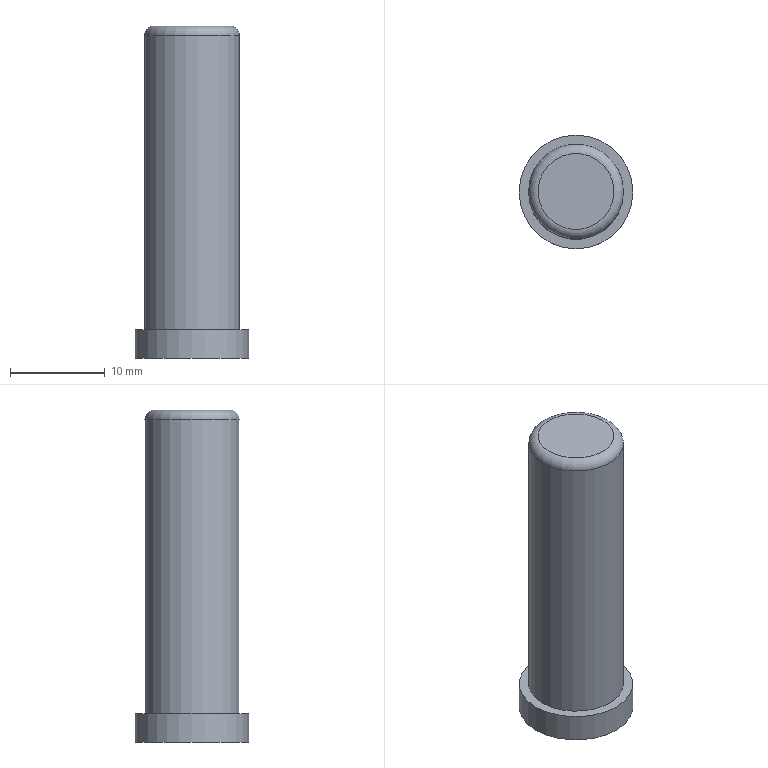Part | NX | features PG_666 2 | 1 solid | 6 faces | box 12 x 12 x 35 mm | volume 2847 mm3 | plane 3 | cylinder 2 | torus 1 | commonest cylinder face diameters 10.001 x1 12 x1
STEP:
#1=CARTESIAN_POINT('',(3665.089,-892.101,822.716));
#2=VERTEX_POINT('',#1);
#3=CARTESIAN_POINT('',(3660.088,-892.101,822.716));
#4=DIRECTION('',(0.,0.,1.));
#5=DIRECTION('',(1.,0.,0.));
#6=AXIS2_PLACEMENT_3D('',#3,#4,#5);
#7=CIRCLE('',#6,5.);
#8=EDGE_CURVE('',#2,#2,#7,.F.);
#9=ORIENTED_EDGE('',*,*,#8,.T.);
#10=EDGE_LOOP('',(#9));
#11=FACE_BOUND('',#10,.T.);
#12=CARTESIAN_POINT('',(3665.089,-892.101,791.716));
#13=VERTEX_POINT('',#12);
#14=CARTESIAN_POINT('',(3660.088,-892.101,791.716));
#15=DIRECTION('',(0.,0.,1.));
#16=DIRECTION('',(1.,0.,0.));
#17=AXIS2_PLACEMENT_3D('',#14,#15,#16);
#18=CIRCLE('',#17,5.);
#19=EDGE_CURVE('',#13,#13,#18,.F.);
#20=ORIENTED_EDGE('',*,*,#19,.F.);
#21=EDGE_LOOP('',(#20));
#22=FACE_BOUND('',#21,.T.);
#23=CARTESIAN_POINT('',(3660.088,-892.101,811.716));
#24=DIRECTION('',(0.,0.,-1.));
#25=DIRECTION('',(-1.,0.,0.));
#26=AXIS2_PLACEMENT_3D('',#23,#24,#25);
#27=CYLINDRICAL_SURFACE('',#26,5.);
#28=ADVANCED_FACE('',(#11,#22),#27,.T.);
#29=CARTESIAN_POINT('',(3664.089,-892.101,823.716));
#30=VERTEX_POINT('',#29);
#31=CARTESIAN_POINT('',(3660.088,-892.101,823.716));
#32=DIRECTION('',(0.,0.,1.));
#33=DIRECTION('',(1.,0.,0.));
#34=AXIS2_PLACEMENT_3D('',#31,#32,#33);
#35=CIRCLE('',#34,4.);
#36=EDGE_CURVE('',#30,#30,#35,.T.);
#37=ORIENTED_EDGE('',*,*,#36,.T.);
#38=EDGE_LOOP('',(#37));
#39=FACE_BOUND('',#38,.T.);
#40=CARTESIAN_POINT('',(3660.088,-892.101,823.716));
#41=DIRECTION('',(0.,0.,1.));
#42=DIRECTION('',(1.,0.,0.));
#43=AXIS2_PLACEMENT_3D('',#40,#41,#42);
#44=PLANE('',#43);
#45=ADVANCED_FACE('',(#39),#44,.T.);
#46=CARTESIAN_POINT('',(3654.088,-892.101,788.716));
#47=VERTEX_POINT('',#46);
#48=CARTESIAN_POINT('',(3660.088,-892.101,788.716));
#49=DIRECTION('',(0.,0.,1.));
#50=DIRECTION('',(-1.,0.,0.));
#51=AXIS2_PLACEMENT_3D('',#48,#49,#50);
#52=CIRCLE('',#51,6.);
#53=EDGE_CURVE('',#47,#47,#52,.T.);
#54=ORIENTED_EDGE('',*,*,#53,.F.);
#55=EDGE_LOOP('',(#54));
#56=FACE_BOUND('',#55,.T.);
#57=CARTESIAN_POINT('',(3660.088,-892.101,788.716));
#58=DIRECTION('',(0.,0.,-1.));
#59=DIRECTION('',(-1.,0.,0.));
#60=AXIS2_PLACEMENT_3D('',#57,#58,#59);
#61=PLANE('',#60);
#62=ADVANCED_FACE('',(#56),#61,.T.);
#63=ORIENTED_EDGE('',*,*,#19,.T.);
#64=EDGE_LOOP('',(#63));
#65=FACE_BOUND('',#64,.T.);
#66=CARTESIAN_POINT('',(3654.088,-892.101,791.716));
#67=VERTEX_POINT('',#66);
#68=CARTESIAN_POINT('',(3660.088,-892.101,791.716));
#69=DIRECTION('',(0.,0.,-1.));
#70=DIRECTION('',(-1.,0.,0.));
#71=AXIS2_PLACEMENT_3D('',#68,#69,#70);
#72=CIRCLE('',#71,6.);
#73=EDGE_CURVE('',#67,#67,#72,.T.);
#74=ORIENTED_EDGE('',*,*,#73,.F.);
#75=EDGE_LOOP('',(#74));
#76=FACE_BOUND('',#75,.T.);
#77=CARTESIAN_POINT('',(3660.088,-892.101,791.716));
#78=DIRECTION('',(0.,0.,1.));
#79=DIRECTION('',(1.,0.,0.));
#80=AXIS2_PLACEMENT_3D('',#77,#78,#79);
#81=PLANE('',#80);
#82=ADVANCED_FACE('',(#65,#76),#81,.T.);
#83=ORIENTED_EDGE('',*,*,#53,.T.);
#84=EDGE_LOOP('',(#83));
#85=FACE_BOUND('',#84,.T.);
#86=ORIENTED_EDGE('',*,*,#73,.T.);
#87=EDGE_LOOP('',(#86));
#88=FACE_BOUND('',#87,.T.);
#89=CARTESIAN_POINT('',(3660.088,-892.101,791.716));
#90=DIRECTION('',(0.,0.,-1.));
#91=DIRECTION('',(-1.,0.,0.));
#92=AXIS2_PLACEMENT_3D('',#89,#90,#91);
#93=CYLINDRICAL_SURFACE('',#92,6.);
#94=ADVANCED_FACE('',(#85,#88),#93,.T.);
#95=ORIENTED_EDGE('',*,*,#36,.F.);
#96=EDGE_LOOP('',(#95));
#97=FACE_BOUND('',#96,.T.);
#98=ORIENTED_EDGE('',*,*,#8,.F.);
#99=EDGE_LOOP('',(#98));
#100=FACE_BOUND('',#99,.T.);
#101=CARTESIAN_POINT('',(3660.088,-892.101,822.716));
#102=DIRECTION('',(0.,0.,1.));
#103=DIRECTION('',(1.,0.,0.));
#104=AXIS2_PLACEMENT_3D('',#101,#102,#103);
#105=TOROIDAL_SURFACE('',#104,4.,1.);
#106=ADVANCED_FACE('',(#97,#100),#105,.T.);
#107=CLOSED_SHELL('',(#28,#45,#62,#82,#94,#106));
#108=MANIFOLD_SOLID_BREP('',#107);
#109=(LENGTH_UNIT()NAMED_UNIT(*)SI_UNIT(.MILLI.,.METRE.));
#110=UNCERTAINTY_MEASURE_WITH_UNIT(LENGTH_MEASURE(0.00001),#109,'','');
#111=(NAMED_UNIT(*)PLANE_ANGLE_UNIT()SI_UNIT($,.RADIAN.));
#112=(NAMED_UNIT(*)SI_UNIT($,.STERADIAN.)SOLID_ANGLE_UNIT());
#113=(GEOMETRIC_REPRESENTATION_CONTEXT(3)GLOBAL_UNCERTAINTY_ASSIGNED_CONTEXT((#110))GLOBAL_UNIT_ASSIGNED_CONTEXT((#109,#111,#112))REPRESENTATION_CONTEXT('',''));
#114=ADVANCED_BREP_SHAPE_REPRESENTATION('',(#108),#113);